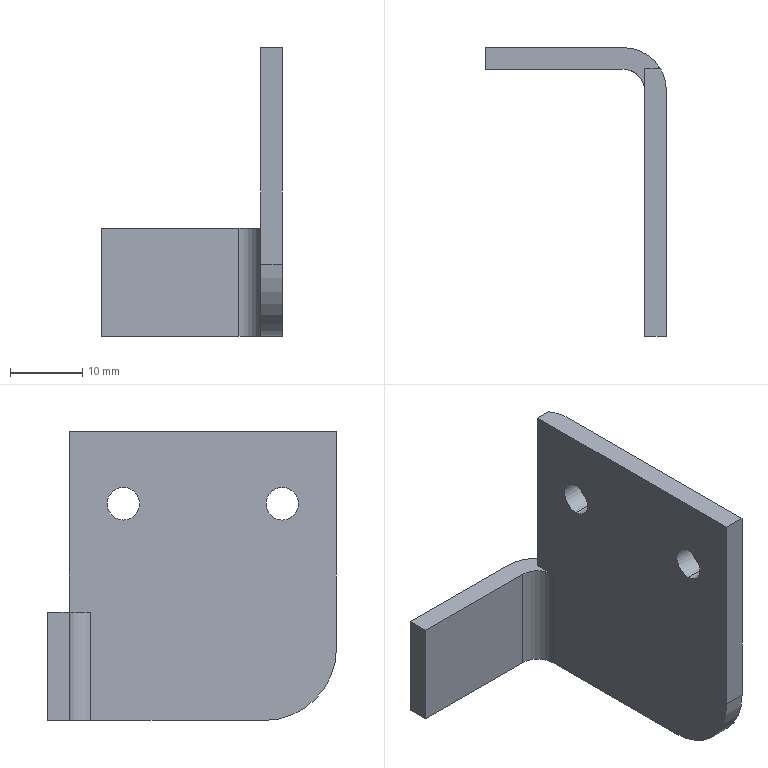Part | STEP file | X77-04018 | 1 solid | 17 faces | box 25 x 40 x 40 mm | volume 5299 mm3 | plane 10 | cylinder 7 | commonest cylinder face diameters 4.5 x4 6 x1 12 x1 20 x1
STEP:
#1=CARTESIAN_POINT('',(-36.443,201.927,32.25));
#2=VERTEX_POINT('',#1);
#3=CARTESIAN_POINT('',(-36.443,201.927,27.75));
#4=VERTEX_POINT('',#3);
#5=CARTESIAN_POINT('',(-36.443,201.927,30.));
#6=DIRECTION('',(1.,0.,0.));
#7=DIRECTION('',(0.,1.,0.));
#8=AXIS2_PLACEMENT_3D('',#5,#6,#7);
#9=CIRCLE('',#8,2.25);
#10=EDGE_CURVE('',#2,#4,#9,.T.);
#11=ORIENTED_EDGE('',*,*,#10,.F.);
#12=CARTESIAN_POINT('',(-33.443,201.927,32.25));
#13=VERTEX_POINT('',#12);
#14=CARTESIAN_POINT('',(-58.443,201.927,32.25));
#15=DIRECTION('',(1.,0.,0.));
#16=VECTOR('',#15,1000.);
#17=LINE('',#14,#16);
#18=EDGE_CURVE('',#2,#13,#17,.T.);
#19=ORIENTED_EDGE('',*,*,#18,.T.);
#20=CARTESIAN_POINT('',(-33.443,201.927,27.75));
#21=VERTEX_POINT('',#20);
#22=CARTESIAN_POINT('',(-33.443,201.927,30.));
#23=DIRECTION('',(1.,0.,0.));
#24=DIRECTION('',(0.,0.,-1.));
#25=AXIS2_PLACEMENT_3D('',#22,#23,#24);
#26=CIRCLE('',#25,2.25);
#27=EDGE_CURVE('',#13,#21,#26,.T.);
#28=ORIENTED_EDGE('',*,*,#27,.T.);
#29=CARTESIAN_POINT('',(-58.443,201.927,27.75));
#30=DIRECTION('',(1.,0.,0.));
#31=VECTOR('',#30,1000.);
#32=LINE('',#29,#31);
#33=EDGE_CURVE('',#4,#21,#32,.T.);
#34=ORIENTED_EDGE('',*,*,#33,.F.);
#35=EDGE_LOOP('',(#11,#19,#28,#34));
#36=FACE_OUTER_BOUND('',#35,.T.);
#37=CARTESIAN_POINT('',(-58.443,201.927,30.));
#38=DIRECTION('',(1.,0.,0.));
#39=DIRECTION('',(0.,0.,-1.));
#40=AXIS2_PLACEMENT_3D('',#37,#38,#39);
#41=CYLINDRICAL_SURFACE('',#40,2.25);
#42=ADVANCED_FACE('',(#36),#41,.F.);
#43=CARTESIAN_POINT('',(-36.443,179.927,32.25));
#44=VERTEX_POINT('',#43);
#45=CARTESIAN_POINT('',(-36.443,179.927,27.75));
#46=VERTEX_POINT('',#45);
#47=CARTESIAN_POINT('',(-36.443,179.927,30.));
#48=DIRECTION('',(1.,0.,0.));
#49=DIRECTION('',(0.,1.,0.));
#50=AXIS2_PLACEMENT_3D('',#47,#48,#49);
#51=CIRCLE('',#50,2.25);
#52=EDGE_CURVE('',#44,#46,#51,.T.);
#53=ORIENTED_EDGE('',*,*,#52,.F.);
#54=CARTESIAN_POINT('',(-33.443,179.927,32.25));
#55=VERTEX_POINT('',#54);
#56=CARTESIAN_POINT('',(-58.443,179.927,32.25));
#57=DIRECTION('',(1.,0.,0.));
#58=VECTOR('',#57,1000.);
#59=LINE('',#56,#58);
#60=EDGE_CURVE('',#44,#55,#59,.T.);
#61=ORIENTED_EDGE('',*,*,#60,.T.);
#62=CARTESIAN_POINT('',(-33.443,179.927,27.75));
#63=VERTEX_POINT('',#62);
#64=CARTESIAN_POINT('',(-33.443,179.927,30.));
#65=DIRECTION('',(1.,0.,0.));
#66=DIRECTION('',(0.,0.,-1.));
#67=AXIS2_PLACEMENT_3D('',#64,#65,#66);
#68=CIRCLE('',#67,2.25);
#69=EDGE_CURVE('',#55,#63,#68,.T.);
#70=ORIENTED_EDGE('',*,*,#69,.T.);
#71=CARTESIAN_POINT('',(-58.443,179.927,27.75));
#72=DIRECTION('',(1.,0.,0.));
#73=VECTOR('',#72,1000.);
#74=LINE('',#71,#73);
#75=EDGE_CURVE('',#46,#63,#74,.T.);
#76=ORIENTED_EDGE('',*,*,#75,.F.);
#77=EDGE_LOOP('',(#53,#61,#70,#76));
#78=FACE_OUTER_BOUND('',#77,.T.);
#79=CARTESIAN_POINT('',(-58.443,179.927,30.));
#80=DIRECTION('',(1.,0.,0.));
#81=DIRECTION('',(0.,0.,-1.));
#82=AXIS2_PLACEMENT_3D('',#79,#80,#81);
#83=CYLINDRICAL_SURFACE('',#82,2.25);
#84=ADVANCED_FACE('',(#78),#83,.F.);
#85=CARTESIAN_POINT('',(-33.443,172.427,40.));
#86=VERTEX_POINT('',#85);
#87=CARTESIAN_POINT('',(-33.443,206.427,40.));
#88=VERTEX_POINT('',#87);
#89=CARTESIAN_POINT('',(-33.443,172.427,40.));
#90=DIRECTION('',(0.,1.,0.));
#91=VECTOR('',#90,1000.);
#92=LINE('',#89,#91);
#93=EDGE_CURVE('',#86,#88,#92,.T.);
#94=ORIENTED_EDGE('',*,*,#93,.T.);
#95=CARTESIAN_POINT('',(-34.246,209.427,40.));
#96=VERTEX_POINT('',#95);
#97=CARTESIAN_POINT('',(-39.443,206.427,40.));
#98=DIRECTION('',(0.,0.,1.));
#99=DIRECTION('',(1.,0.,0.));
#100=AXIS2_PLACEMENT_3D('',#97,#98,#99);
#101=CIRCLE('',#100,6.);
#102=EDGE_CURVE('',#88,#96,#101,.T.);
#103=ORIENTED_EDGE('',*,*,#102,.T.);
#104=CARTESIAN_POINT('',(-36.443,209.427,40.));
#105=VERTEX_POINT('',#104);
#106=CARTESIAN_POINT('',(-58.443,209.427,40.));
#107=DIRECTION('',(-1.,0.,0.));
#108=VECTOR('',#107,1000.);
#109=LINE('',#106,#108);
#110=EDGE_CURVE('',#96,#105,#109,.T.);
#111=ORIENTED_EDGE('',*,*,#110,.T.);
#112=CARTESIAN_POINT('',(-36.443,172.427,40.));
#113=VERTEX_POINT('',#112);
#114=CARTESIAN_POINT('',(-36.443,209.427,40.));
#115=DIRECTION('',(0.,-1.,0.));
#116=VECTOR('',#115,1000.);
#117=LINE('',#114,#116);
#118=EDGE_CURVE('',#105,#113,#117,.T.);
#119=ORIENTED_EDGE('',*,*,#118,.T.);
#120=CARTESIAN_POINT('',(-36.443,172.427,40.));
#121=DIRECTION('',(1.,0.,0.));
#122=VECTOR('',#121,1000.);
#123=LINE('',#120,#122);
#124=EDGE_CURVE('',#113,#86,#123,.T.);
#125=ORIENTED_EDGE('',*,*,#124,.T.);
#126=EDGE_LOOP('',(#94,#103,#111,#119,#125));
#127=FACE_OUTER_BOUND('',#126,.T.);
#128=CARTESIAN_POINT('',(-33.443,212.427,40.));
#129=DIRECTION('',(0.,0.,1.));
#130=DIRECTION('',(1.,0.,0.));
#131=AXIS2_PLACEMENT_3D('',#128,#129,#130);
#132=PLANE('',#131);
#133=ADVANCED_FACE('',(#127),#132,.T.);
#134=CARTESIAN_POINT('',(-33.443,201.927,30.));
#135=DIRECTION('',(1.,0.,0.));
#136=DIRECTION('',(0.,0.,-1.));
#137=AXIS2_PLACEMENT_3D('',#134,#135,#136);
#138=CIRCLE('',#137,2.25);
#139=EDGE_CURVE('',#21,#13,#138,.T.);
#140=ORIENTED_EDGE('',*,*,#139,.F.);
#141=ORIENTED_EDGE('',*,*,#27,.F.);
#142=EDGE_LOOP('',(#140,#141));
#143=FACE_BOUND('',#142,.T.);
#144=CARTESIAN_POINT('',(-33.443,179.927,30.));
#145=DIRECTION('',(1.,0.,0.));
#146=DIRECTION('',(0.,0.,-1.));
#147=AXIS2_PLACEMENT_3D('',#144,#145,#146);
#148=CIRCLE('',#147,2.25);
#149=EDGE_CURVE('',#63,#55,#148,.T.);
#150=ORIENTED_EDGE('',*,*,#149,.F.);
#151=ORIENTED_EDGE('',*,*,#69,.F.);
#152=EDGE_LOOP('',(#150,#151));
#153=FACE_BOUND('',#152,.T.);
#154=CARTESIAN_POINT('',(-33.443,182.427,0.));
#155=VERTEX_POINT('',#154);
#156=CARTESIAN_POINT('',(-33.443,206.427,0.));
#157=VERTEX_POINT('',#156);
#158=CARTESIAN_POINT('',(-33.443,172.427,0.));
#159=DIRECTION('',(0.,1.,0.));
#160=VECTOR('',#159,1000.);
#161=LINE('',#158,#160);
#162=EDGE_CURVE('',#155,#157,#161,.T.);
#163=ORIENTED_EDGE('',*,*,#162,.T.);
#164=CARTESIAN_POINT('',(-33.443,206.427,40.));
#165=DIRECTION('',(0.,0.,1.));
#166=VECTOR('',#165,1000.);
#167=LINE('',#164,#166);
#168=EDGE_CURVE('',#157,#88,#167,.T.);
#169=ORIENTED_EDGE('',*,*,#168,.T.);
#170=ORIENTED_EDGE('',*,*,#93,.F.);
#171=CARTESIAN_POINT('',(-33.443,172.427,10.));
#172=VERTEX_POINT('',#171);
#173=CARTESIAN_POINT('',(-33.443,172.427,40.));
#174=DIRECTION('',(0.,0.,-1.));
#175=VECTOR('',#174,1000.);
#176=LINE('',#173,#175);
#177=EDGE_CURVE('',#86,#172,#176,.T.);
#178=ORIENTED_EDGE('',*,*,#177,.T.);
#179=CARTESIAN_POINT('',(-33.443,182.427,10.));
#180=DIRECTION('',(1.,0.,0.));
#181=DIRECTION('',(0.,0.,1.));
#182=AXIS2_PLACEMENT_3D('',#179,#180,#181);
#183=CIRCLE('',#182,10.);
#184=EDGE_CURVE('',#172,#155,#183,.T.);
#185=ORIENTED_EDGE('',*,*,#184,.T.);
#186=EDGE_LOOP('',(#163,#169,#170,#178,#185));
#187=FACE_OUTER_BOUND('',#186,.T.);
#188=CARTESIAN_POINT('',(-33.443,172.427,40.));
#189=DIRECTION('',(-1.,0.,0.));
#190=DIRECTION('',(0.,0.,1.));
#191=AXIS2_PLACEMENT_3D('',#188,#189,#190);
#192=PLANE('',#191);
#193=ADVANCED_FACE('',(#143,#153,#187),#192,.F.);
#194=CARTESIAN_POINT('',(-58.443,212.427,15.));
#195=VERTEX_POINT('',#194);
#196=CARTESIAN_POINT('',(-39.443,212.427,15.));
#197=VERTEX_POINT('',#196);
#198=CARTESIAN_POINT('',(-58.443,212.427,15.));
#199=DIRECTION('',(1.,0.,0.));
#200=VECTOR('',#199,1000.);
#201=LINE('',#198,#200);
#202=EDGE_CURVE('',#195,#197,#201,.T.);
#203=ORIENTED_EDGE('',*,*,#202,.T.);
#204=CARTESIAN_POINT('',(-39.443,212.427,0.));
#205=VERTEX_POINT('',#204);
#206=CARTESIAN_POINT('',(-39.443,212.427,40.));
#207=DIRECTION('',(0.,0.,-1.));
#208=VECTOR('',#207,1000.);
#209=LINE('',#206,#208);
#210=EDGE_CURVE('',#197,#205,#209,.T.);
#211=ORIENTED_EDGE('',*,*,#210,.T.);
#212=CARTESIAN_POINT('',(-58.443,212.427,0.));
#213=VERTEX_POINT('',#212);
#214=CARTESIAN_POINT('',(-33.443,212.427,0.));
#215=DIRECTION('',(-1.,0.,0.));
#216=VECTOR('',#215,1000.);
#217=LINE('',#214,#216);
#218=EDGE_CURVE('',#205,#213,#217,.T.);
#219=ORIENTED_EDGE('',*,*,#218,.T.);
#220=CARTESIAN_POINT('',(-58.443,212.427,40.));
#221=DIRECTION('',(0.,0.,-1.));
#222=VECTOR('',#221,1000.);
#223=LINE('',#220,#222);
#224=EDGE_CURVE('',#195,#213,#223,.T.);
#225=ORIENTED_EDGE('',*,*,#224,.F.);
#226=EDGE_LOOP('',(#203,#211,#219,#225));
#227=FACE_OUTER_BOUND('',#226,.T.);
#228=CARTESIAN_POINT('',(-33.443,212.427,40.));
#229=DIRECTION('',(0.,-1.,0.));
#230=DIRECTION('',(0.,0.,-1.));
#231=AXIS2_PLACEMENT_3D('',#228,#229,#230);
#232=PLANE('',#231);
#233=ADVANCED_FACE('',(#227),#232,.F.);
#234=CARTESIAN_POINT('',(-58.443,209.427,15.));
#235=VERTEX_POINT('',#234);
#236=CARTESIAN_POINT('',(-58.443,209.427,0.));
#237=VERTEX_POINT('',#236);
#238=CARTESIAN_POINT('',(-58.443,209.427,40.));
#239=DIRECTION('',(0.,0.,-1.));
#240=VECTOR('',#239,1000.);
#241=LINE('',#238,#240);
#242=EDGE_CURVE('',#235,#237,#241,.T.);
#243=ORIENTED_EDGE('',*,*,#242,.F.);
#244=CARTESIAN_POINT('',(-58.443,212.427,15.));
#245=DIRECTION('',(0.,-1.,0.));
#246=VECTOR('',#245,1000.);
#247=LINE('',#244,#246);
#248=EDGE_CURVE('',#195,#235,#247,.T.);
#249=ORIENTED_EDGE('',*,*,#248,.F.);
#250=ORIENTED_EDGE('',*,*,#224,.T.);
#251=CARTESIAN_POINT('',(-58.443,212.427,0.));
#252=DIRECTION('',(0.,-1.,0.));
#253=VECTOR('',#252,1000.);
#254=LINE('',#251,#253);
#255=EDGE_CURVE('',#213,#237,#254,.T.);
#256=ORIENTED_EDGE('',*,*,#255,.T.);
#257=EDGE_LOOP('',(#243,#249,#250,#256));
#258=FACE_OUTER_BOUND('',#257,.T.);
#259=CARTESIAN_POINT('',(-58.443,212.427,40.));
#260=DIRECTION('',(1.,0.,0.));
#261=DIRECTION('',(0.,0.,-1.));
#262=AXIS2_PLACEMENT_3D('',#259,#260,#261);
#263=PLANE('',#262);
#264=ADVANCED_FACE('',(#258),#263,.F.);
#265=CARTESIAN_POINT('',(-39.443,209.427,0.));
#266=VERTEX_POINT('',#265);
#267=CARTESIAN_POINT('',(-58.443,209.427,0.));
#268=DIRECTION('',(1.,0.,0.));
#269=VECTOR('',#268,1000.);
#270=LINE('',#267,#269);
#271=EDGE_CURVE('',#237,#266,#270,.T.);
#272=ORIENTED_EDGE('',*,*,#271,.T.);
#273=CARTESIAN_POINT('',(-39.443,209.427,15.));
#274=VERTEX_POINT('',#273);
#275=CARTESIAN_POINT('',(-39.443,209.427,15.));
#276=DIRECTION('',(0.,0.,1.));
#277=VECTOR('',#276,1000.);
#278=LINE('',#275,#277);
#279=EDGE_CURVE('',#266,#274,#278,.T.);
#280=ORIENTED_EDGE('',*,*,#279,.T.);
#281=CARTESIAN_POINT('',(-58.443,209.427,15.));
#282=DIRECTION('',(1.,0.,0.));
#283=VECTOR('',#282,1000.);
#284=LINE('',#281,#283);
#285=EDGE_CURVE('',#235,#274,#284,.T.);
#286=ORIENTED_EDGE('',*,*,#285,.F.);
#287=ORIENTED_EDGE('',*,*,#242,.T.);
#288=EDGE_LOOP('',(#272,#280,#286,#287));
#289=FACE_OUTER_BOUND('',#288,.T.);
#290=CARTESIAN_POINT('',(-58.443,209.427,40.));
#291=DIRECTION('',(0.,1.,0.));
#292=DIRECTION('',(0.,0.,1.));
#293=AXIS2_PLACEMENT_3D('',#290,#291,#292);
#294=PLANE('',#293);
#295=ADVANCED_FACE('',(#289),#294,.F.);
#296=CARTESIAN_POINT('',(-36.443,201.927,30.));
#297=DIRECTION('',(1.,0.,0.));
#298=DIRECTION('',(0.,1.,0.));
#299=AXIS2_PLACEMENT_3D('',#296,#297,#298);
#300=CIRCLE('',#299,2.25);
#301=EDGE_CURVE('',#4,#2,#300,.T.);
#302=ORIENTED_EDGE('',*,*,#301,.T.);
#303=ORIENTED_EDGE('',*,*,#10,.T.);
#304=EDGE_LOOP('',(#302,#303));
#305=FACE_BOUND('',#304,.T.);
#306=CARTESIAN_POINT('',(-36.443,179.927,30.));
#307=DIRECTION('',(1.,0.,0.));
#308=DIRECTION('',(0.,1.,0.));
#309=AXIS2_PLACEMENT_3D('',#306,#307,#308);
#310=CIRCLE('',#309,2.25);
#311=EDGE_CURVE('',#46,#44,#310,.T.);
#312=ORIENTED_EDGE('',*,*,#311,.T.);
#313=ORIENTED_EDGE('',*,*,#52,.T.);
#314=EDGE_LOOP('',(#312,#313));
#315=FACE_BOUND('',#314,.T.);
#316=CARTESIAN_POINT('',(-36.443,209.427,15.));
#317=VERTEX_POINT('',#316);
#318=CARTESIAN_POINT('',(-36.443,206.427,15.));
#319=VERTEX_POINT('',#318);
#320=CARTESIAN_POINT('',(-36.443,212.427,15.));
#321=DIRECTION('',(0.,-1.,0.));
#322=VECTOR('',#321,1000.);
#323=LINE('',#320,#322);
#324=EDGE_CURVE('',#317,#319,#323,.T.);
#325=ORIENTED_EDGE('',*,*,#324,.T.);
#326=CARTESIAN_POINT('',(-36.443,206.427,0.));
#327=VERTEX_POINT('',#326);
#328=CARTESIAN_POINT('',(-36.443,206.427,0.));
#329=DIRECTION('',(0.,0.,-1.));
#330=VECTOR('',#329,1000.);
#331=LINE('',#328,#330);
#332=EDGE_CURVE('',#319,#327,#331,.T.);
#333=ORIENTED_EDGE('',*,*,#332,.T.);
#334=CARTESIAN_POINT('',(-36.443,182.427,0.));
#335=VERTEX_POINT('',#334);
#336=CARTESIAN_POINT('',(-36.443,209.427,0.));
#337=DIRECTION('',(0.,-1.,0.));
#338=VECTOR('',#337,1000.);
#339=LINE('',#336,#338);
#340=EDGE_CURVE('',#327,#335,#339,.T.);
#341=ORIENTED_EDGE('',*,*,#340,.T.);
#342=CARTESIAN_POINT('',(-36.443,172.427,10.));
#343=VERTEX_POINT('',#342);
#344=CARTESIAN_POINT('',(-36.443,182.427,10.));
#345=DIRECTION('',(-1.,0.,0.));
#346=DIRECTION('',(0.,1.,0.));
#347=AXIS2_PLACEMENT_3D('',#344,#345,#346);
#348=CIRCLE('',#347,10.);
#349=EDGE_CURVE('',#335,#343,#348,.T.);
#350=ORIENTED_EDGE('',*,*,#349,.T.);
#351=CARTESIAN_POINT('',(-36.443,172.427,40.));
#352=DIRECTION('',(0.,0.,-1.));
#353=VECTOR('',#352,1000.);
#354=LINE('',#351,#353);
#355=EDGE_CURVE('',#113,#343,#354,.T.);
#356=ORIENTED_EDGE('',*,*,#355,.F.);
#357=ORIENTED_EDGE('',*,*,#118,.F.);
#358=CARTESIAN_POINT('',(-36.443,209.427,40.));
#359=DIRECTION('',(0.,0.,-1.));
#360=VECTOR('',#359,1000.);
#361=LINE('',#358,#360);
#362=EDGE_CURVE('',#105,#317,#361,.T.);
#363=ORIENTED_EDGE('',*,*,#362,.T.);
#364=EDGE_LOOP('',(#325,#333,#341,#350,#356,#357,#363));
#365=FACE_OUTER_BOUND('',#364,.T.);
#366=CARTESIAN_POINT('',(-36.443,209.427,40.));
#367=DIRECTION('',(1.,0.,0.));
#368=DIRECTION('',(0.,1.,0.));
#369=AXIS2_PLACEMENT_3D('',#366,#367,#368);
#370=PLANE('',#369);
#371=ADVANCED_FACE('',(#305,#315,#365),#370,.F.);
#372=ORIENTED_EDGE('',*,*,#355,.T.);
#373=CARTESIAN_POINT('',(-36.443,172.427,10.));
#374=DIRECTION('',(1.,0.,0.));
#375=VECTOR('',#374,1000.);
#376=LINE('',#373,#375);
#377=EDGE_CURVE('',#343,#172,#376,.T.);
#378=ORIENTED_EDGE('',*,*,#377,.T.);
#379=ORIENTED_EDGE('',*,*,#177,.F.);
#380=ORIENTED_EDGE('',*,*,#124,.F.);
#381=EDGE_LOOP('',(#372,#378,#379,#380));
#382=FACE_OUTER_BOUND('',#381,.T.);
#383=CARTESIAN_POINT('',(-36.443,172.427,40.));
#384=DIRECTION('',(0.,1.,0.));
#385=DIRECTION('',(0.,0.,1.));
#386=AXIS2_PLACEMENT_3D('',#383,#384,#385);
#387=PLANE('',#386);
#388=ADVANCED_FACE('',(#382),#387,.F.);
#389=ORIENTED_EDGE('',*,*,#218,.F.);
#390=CARTESIAN_POINT('',(-39.443,206.427,0.));
#391=DIRECTION('',(0.,0.,-1.));
#392=DIRECTION('',(1.,0.,0.));
#393=AXIS2_PLACEMENT_3D('',#390,#391,#392);
#394=CIRCLE('',#393,6.);
#395=EDGE_CURVE('',#205,#157,#394,.T.);
#396=ORIENTED_EDGE('',*,*,#395,.T.);
#397=ORIENTED_EDGE('',*,*,#162,.F.);
#398=CARTESIAN_POINT('',(-33.443,182.427,0.));
#399=DIRECTION('',(-1.,0.,0.));
#400=VECTOR('',#399,1000.);
#401=LINE('',#398,#400);
#402=EDGE_CURVE('',#155,#335,#401,.T.);
#403=ORIENTED_EDGE('',*,*,#402,.T.);
#404=ORIENTED_EDGE('',*,*,#340,.F.);
#405=CARTESIAN_POINT('',(-39.443,206.427,0.));
#406=DIRECTION('',(0.,0.,1.));
#407=DIRECTION('',(1.,0.,0.));
#408=AXIS2_PLACEMENT_3D('',#405,#406,#407);
#409=CIRCLE('',#408,3.);
#410=EDGE_CURVE('',#327,#266,#409,.T.);
#411=ORIENTED_EDGE('',*,*,#410,.T.);
#412=ORIENTED_EDGE('',*,*,#271,.F.);
#413=ORIENTED_EDGE('',*,*,#255,.F.);
#414=EDGE_LOOP('',(#389,#396,#397,#403,#404,#411,#412,#413));
#415=FACE_OUTER_BOUND('',#414,.T.);
#416=CARTESIAN_POINT('',(-33.443,212.427,0.));
#417=DIRECTION('',(0.,0.,1.));
#418=DIRECTION('',(1.,0.,0.));
#419=AXIS2_PLACEMENT_3D('',#416,#417,#418);
#420=PLANE('',#419);
#421=ADVANCED_FACE('',(#415),#420,.F.);
#422=ORIENTED_EDGE('',*,*,#110,.F.);
#423=CARTESIAN_POINT('',(-34.246,209.427,15.));
#424=VERTEX_POINT('',#423);
#425=CARTESIAN_POINT('',(-34.246,209.427,40.));
#426=DIRECTION('',(0.,0.,-1.));
#427=VECTOR('',#426,1000.);
#428=LINE('',#425,#427);
#429=EDGE_CURVE('',#96,#424,#428,.T.);
#430=ORIENTED_EDGE('',*,*,#429,.T.);
#431=CARTESIAN_POINT('',(-58.443,209.427,15.));
#432=DIRECTION('',(1.,0.,0.));
#433=VECTOR('',#432,1000.);
#434=LINE('',#431,#433);
#435=EDGE_CURVE('',#317,#424,#434,.T.);
#436=ORIENTED_EDGE('',*,*,#435,.F.);
#437=ORIENTED_EDGE('',*,*,#362,.F.);
#438=EDGE_LOOP('',(#422,#430,#436,#437));
#439=FACE_OUTER_BOUND('',#438,.T.);
#440=CARTESIAN_POINT('',(-58.443,209.427,40.));
#441=DIRECTION('',(0.,1.,0.));
#442=DIRECTION('',(0.,0.,1.));
#443=AXIS2_PLACEMENT_3D('',#440,#441,#442);
#444=PLANE('',#443);
#445=ADVANCED_FACE('',(#439),#444,.T.);
#446=ORIENTED_EDGE('',*,*,#435,.T.);
#447=CARTESIAN_POINT('',(-39.443,206.427,15.));
#448=DIRECTION('',(0.,0.,1.));
#449=DIRECTION('',(-1.,0.,0.));
#450=AXIS2_PLACEMENT_3D('',#447,#448,#449);
#451=CIRCLE('',#450,6.);
#452=EDGE_CURVE('',#424,#197,#451,.T.);
#453=ORIENTED_EDGE('',*,*,#452,.T.);
#454=ORIENTED_EDGE('',*,*,#202,.F.);
#455=ORIENTED_EDGE('',*,*,#248,.T.);
#456=ORIENTED_EDGE('',*,*,#285,.T.);
#457=CARTESIAN_POINT('',(-39.443,206.427,15.));
#458=DIRECTION('',(0.,0.,-1.));
#459=DIRECTION('',(-1.,0.,0.));
#460=AXIS2_PLACEMENT_3D('',#457,#458,#459);
#461=CIRCLE('',#460,3.);
#462=EDGE_CURVE('',#274,#319,#461,.T.);
#463=ORIENTED_EDGE('',*,*,#462,.T.);
#464=ORIENTED_EDGE('',*,*,#324,.F.);
#465=EDGE_LOOP('',(#446,#453,#454,#455,#456,#463,#464));
#466=FACE_OUTER_BOUND('',#465,.T.);
#467=CARTESIAN_POINT('',(-58.443,212.427,15.));
#468=DIRECTION('',(0.,0.,-1.));
#469=DIRECTION('',(-1.,0.,0.));
#470=AXIS2_PLACEMENT_3D('',#467,#468,#469);
#471=PLANE('',#470);
#472=ADVANCED_FACE('',(#466),#471,.F.);
#473=ORIENTED_EDGE('',*,*,#60,.F.);
#474=ORIENTED_EDGE('',*,*,#311,.F.);
#475=ORIENTED_EDGE('',*,*,#75,.T.);
#476=ORIENTED_EDGE('',*,*,#149,.T.);
#477=EDGE_LOOP('',(#473,#474,#475,#476));
#478=FACE_OUTER_BOUND('',#477,.T.);
#479=CARTESIAN_POINT('',(-58.443,179.927,30.));
#480=DIRECTION('',(1.,0.,0.));
#481=DIRECTION('',(0.,0.,-1.));
#482=AXIS2_PLACEMENT_3D('',#479,#480,#481);
#483=CYLINDRICAL_SURFACE('',#482,2.25);
#484=ADVANCED_FACE('',(#478),#483,.F.);
#485=ORIENTED_EDGE('',*,*,#18,.F.);
#486=ORIENTED_EDGE('',*,*,#301,.F.);
#487=ORIENTED_EDGE('',*,*,#33,.T.);
#488=ORIENTED_EDGE('',*,*,#139,.T.);
#489=EDGE_LOOP('',(#485,#486,#487,#488));
#490=FACE_OUTER_BOUND('',#489,.T.);
#491=CARTESIAN_POINT('',(-58.443,201.927,30.));
#492=DIRECTION('',(1.,0.,0.));
#493=DIRECTION('',(0.,0.,-1.));
#494=AXIS2_PLACEMENT_3D('',#491,#492,#493);
#495=CYLINDRICAL_SURFACE('',#494,2.25);
#496=ADVANCED_FACE('',(#490),#495,.F.);
#497=ORIENTED_EDGE('',*,*,#349,.F.);
#498=ORIENTED_EDGE('',*,*,#402,.F.);
#499=ORIENTED_EDGE('',*,*,#184,.F.);
#500=ORIENTED_EDGE('',*,*,#377,.F.);
#501=EDGE_LOOP('',(#497,#498,#499,#500));
#502=FACE_OUTER_BOUND('',#501,.T.);
#503=CARTESIAN_POINT('',(-36.443,182.427,10.));
#504=DIRECTION('',(1.,0.,0.));
#505=DIRECTION('',(0.,0.,-1.));
#506=AXIS2_PLACEMENT_3D('',#503,#504,#505);
#507=CYLINDRICAL_SURFACE('',#506,10.);
#508=ADVANCED_FACE('',(#502),#507,.T.);
#509=ORIENTED_EDGE('',*,*,#462,.F.);
#510=ORIENTED_EDGE('',*,*,#279,.F.);
#511=ORIENTED_EDGE('',*,*,#410,.F.);
#512=ORIENTED_EDGE('',*,*,#332,.F.);
#513=EDGE_LOOP('',(#509,#510,#511,#512));
#514=FACE_OUTER_BOUND('',#513,.T.);
#515=CARTESIAN_POINT('',(-39.443,206.427,40.));
#516=DIRECTION('',(0.,0.,1.));
#517=DIRECTION('',(1.,0.,0.));
#518=AXIS2_PLACEMENT_3D('',#515,#516,#517);
#519=CYLINDRICAL_SURFACE('',#518,3.);
#520=ADVANCED_FACE('',(#514),#519,.F.);
#521=ORIENTED_EDGE('',*,*,#102,.F.);
#522=ORIENTED_EDGE('',*,*,#168,.F.);
#523=ORIENTED_EDGE('',*,*,#395,.F.);
#524=ORIENTED_EDGE('',*,*,#210,.F.);
#525=ORIENTED_EDGE('',*,*,#452,.F.);
#526=ORIENTED_EDGE('',*,*,#429,.F.);
#527=EDGE_LOOP('',(#521,#522,#523,#524,#525,#526));
#528=FACE_OUTER_BOUND('',#527,.T.);
#529=CARTESIAN_POINT('',(-39.443,206.427,40.));
#530=DIRECTION('',(0.,0.,-1.));
#531=DIRECTION('',(-1.,0.,0.));
#532=AXIS2_PLACEMENT_3D('',#529,#530,#531);
#533=CYLINDRICAL_SURFACE('',#532,6.);
#534=ADVANCED_FACE('',(#528),#533,.T.);
#535=CLOSED_SHELL('',(#42,#84,#133,#193,#233,#264,#295,#371,#388,#421,#445,#472,#484,#496,#508,#520,#534));
#536=MANIFOLD_SOLID_BREP('',#535);
#537=CARTESIAN_POINT('',(0.,0.,0.));
#538=DIRECTION('',(0.,0.,1.));
#539=DIRECTION('',(1.,0.,0.));
#540=AXIS2_PLACEMENT_3D('',#537,#538,#539);
#541=(LENGTH_UNIT()NAMED_UNIT(*)SI_UNIT(.MILLI.,.METRE.));
#542=UNCERTAINTY_MEASURE_WITH_UNIT(LENGTH_MEASURE(0.00001),#541,'','');
#543=(NAMED_UNIT(*)PLANE_ANGLE_UNIT()SI_UNIT($,.RADIAN.));
#544=(NAMED_UNIT(*)SI_UNIT($,.STERADIAN.)SOLID_ANGLE_UNIT());
#545=(GEOMETRIC_REPRESENTATION_CONTEXT(3)GLOBAL_UNCERTAINTY_ASSIGNED_CONTEXT((#542))GLOBAL_UNIT_ASSIGNED_CONTEXT((#541,#543,#544))REPRESENTATION_CONTEXT('',''));
#546=ADVANCED_BREP_SHAPE_REPRESENTATION('',(#536,#540),#545);